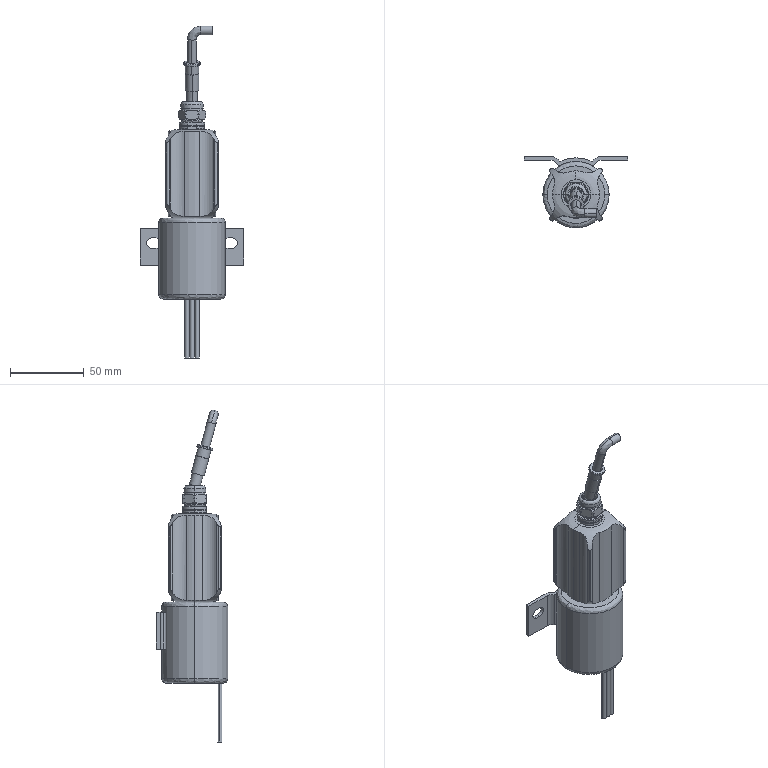Part | SolidWorks | features BaseBody 1 | 1 solid | 200 faces | box 70 x 48.5 x 225.296 mm | volume 154846 mm3 | cylinder 85 | plane 72 | cone 23 | spline 14 | torus 6 | commonest cylinder face diameters 3 x16 18 x10 17.475 x7 7 x6 8 x6 17 x6